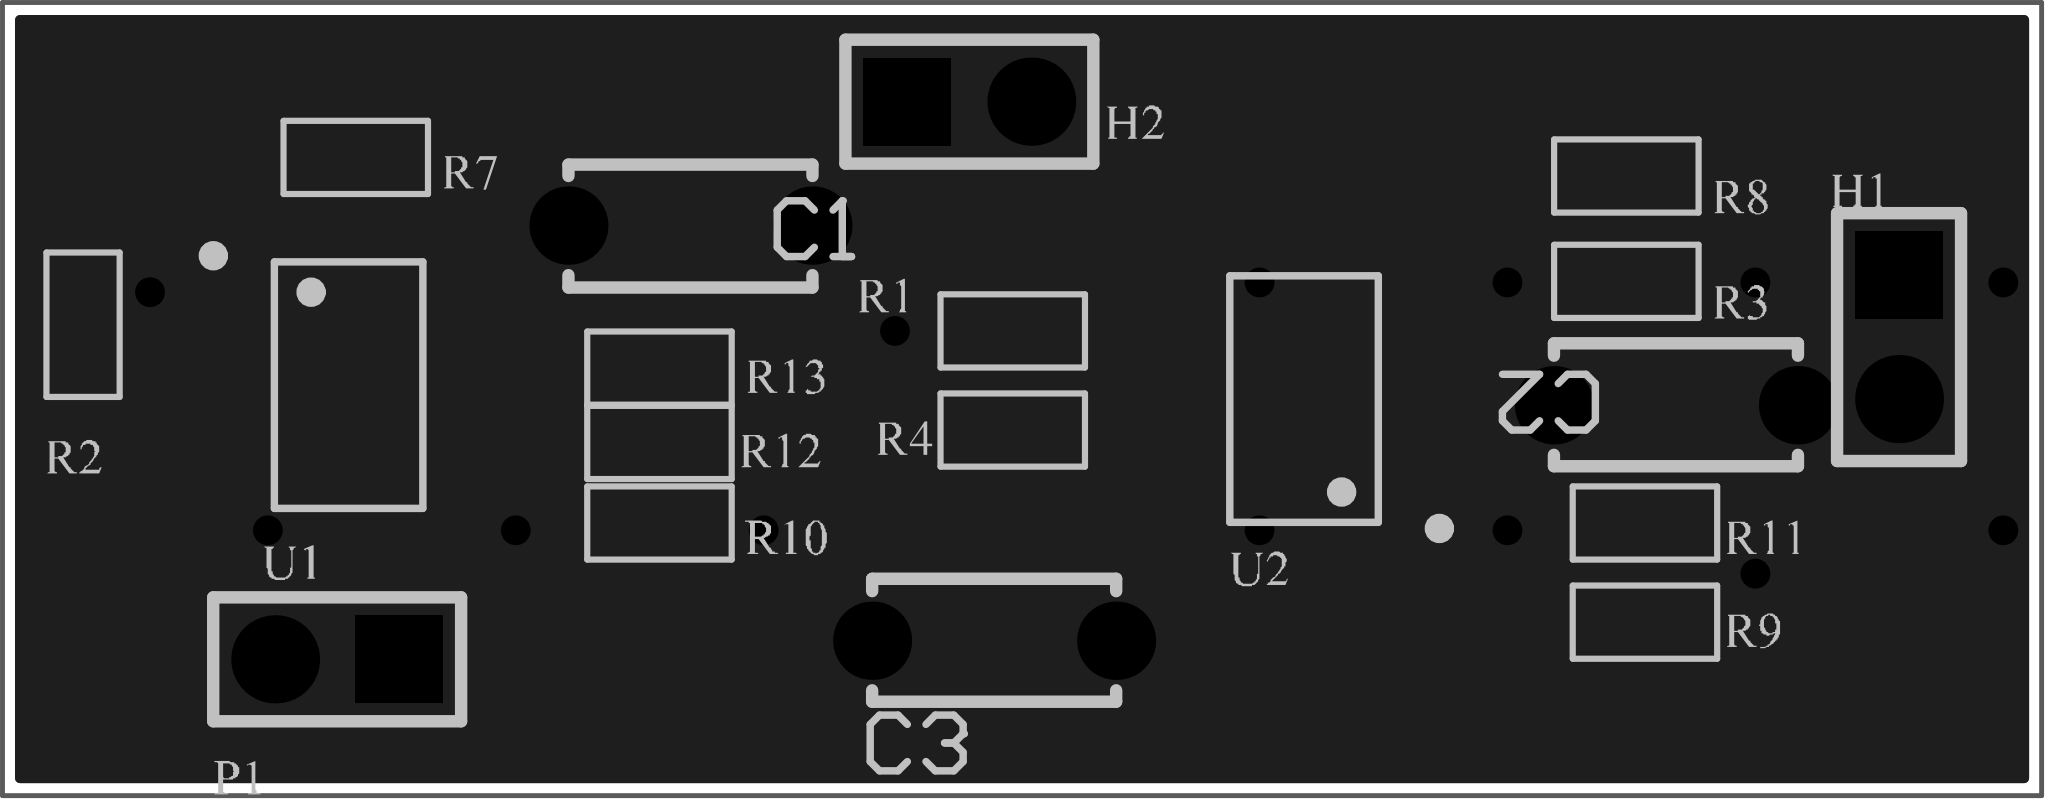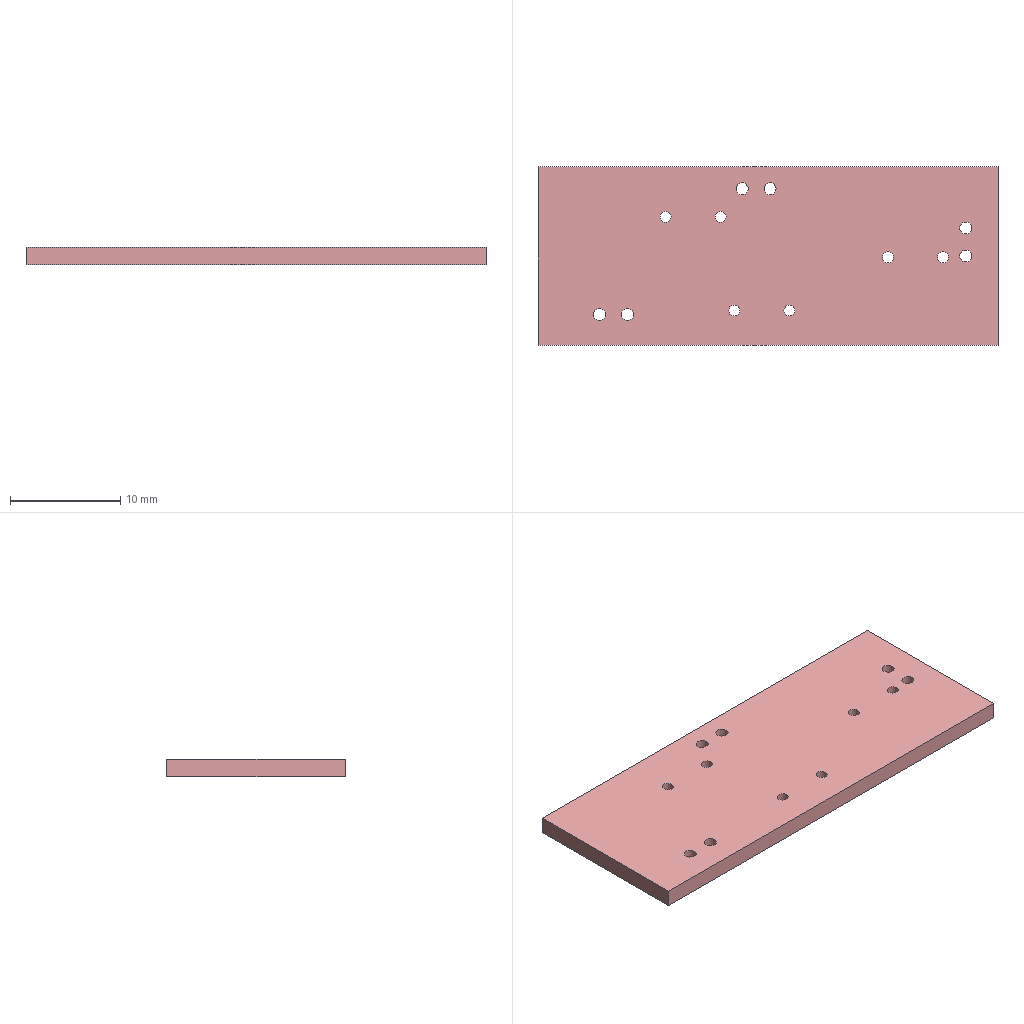Circuit board layout | Altium Designer | box 41.8 x 16.3 x 1.6 mm
Layer stack:
# Altium Designer layer stack of  (unit mm; dielectric type: 0 none, 1 core, 2 prepreg, 3 surface material)
index,name,kind,layer,copper_thickness_mm,dielectric_type,dielectric_thickness_mm,dielectric_material,dielectric_constant
0,Top Paste Mask Layer,other,,,,,,
1,Top Silkscreen Layer,other,,,,,,
2,Top Solder Mask Layer,dielectric,,,3,0.01,,3.3
3,Top Layer,copper,Top Layer,0.035,,,,
4,Dielectric1,dielectric,,,3,1.51,FR4,4.5
5,Bottom Layer,copper,Bottom Layer,0.035,,,,
6,Bottom Solder Mask Layer,dielectric,,,3,0.01,,3.3
7,Bottom Silkscreen Layer,other,,,,,,
8,Bottom Paste Mask Layer,other,,,,,,
# drill layer pairs: low layer,high layer
drill_pair,Top Layer,Bottom Layer
Part placement:
Designator,Comment,Layer,Footprint,Center-X(mm),Center-Y(mm),Rotation
H1,,TopLayer,HDR-TH_2P-P2.54-V-M-1,116.078,88.011,270
H2,,TopLayer,HDR-TH_2P-P2.54-V-M-1,97.028,92.837,0
P1,Header 2,TopLayer,HDR-TH_2P-P2.54-V-M-1,84.074,81.407,180
R1,10K,TopLayer,R0603_SMD-CRCW060327R0FKEA,97.917,88.138,180
R2,10K,TopLayer,R0603_SMD-CRCW060327R0FKEA,78.867,88.265,90
R3,1.22K,TopLayer,R0603_SMD-CRCW060327R0FKEA,110.49,89.154,180
R4,10K,TopLayer,R0603_SMD-CRCW060327R0FKEA,97.917,86.106,180
R7,100,TopLayer,R0603_SMD-CRCW060327R0FKEA,84.455,91.694,180
R8,1.22K,TopLayer,R0603_SMD-CRCW060327R0FKEA,110.49,91.313,0
R9,4.7K,TopLayer,R0603_SMD-CRCW060327R0FKEA,110.871,82.169,0
R10,10K,TopLayer,R0603_SMD-CRCW060327R0FKEA,90.678,84.201,0
R11,4.7K,TopLayer,R0603_SMD-CRCW060327R0FKEA,110.871,84.201,180
R12,10K,TopLayer,R0603_SMD-CRCW060327R0FKEA,90.678,85.852,180
R13,10K,TopLayer,R0603_SMD-CRCW060327R0FKEA,90.678,87.376,180
U1,AD8652ARZ,TopLayer,SOIC-8_L4.9-W3.9-P1.27-LS6.0-BL,84.309,87.027,270
U2,AD8652ARZ,TopLayer,SOIC-8_L4.9-W3.9-P1.27-LS6.0-BL,103.886,86.741,90
C1,Cap,TopLayer,CAP-TH_L5.0-W2.5-P5.00-D1.0,91.313,90.297,0
C2,Cap,TopLayer,CAP-TH_L5.0-W2.5-P5.00-D1.0,111.506,86.614,180
C3,Cap,TopLayer,CAP-TH_L5.0-W2.5-P5.00-D1.0,97.536,81.788,180
Pad and via stacks:
# Altium Designer via and pad stacks of  (unit mm). Each distinct definition once, with the count of objects using it.
# via: kind,start_layer,end_layer,hole_mm,diameter_mm,mode(0 simple;1 top-mid-bottom;2 full stack),diameter_per_layer,count,example_net
# pad: kind,layer,hole_mm,hole_type(0 round;1 square;2 slot),plating,top_size,top_shape(1 round;2 rect;3 octagon;9 rounded rect),mid_size,bottom_size,mode,footprint,size_per_layer,count,example
pad,Multi-Layer,1.1,0,plated,1.8x1.8,1,1.8x1.8,1.8x1.8,0,HDR-TH_2P-P2.54-V-M-1,,3,H1.2
pad,Multi-Layer,1.1,0,plated,1.8x1.8,2,1.8x1.8,1.8x1.8,0,HDR-TH_2P-P2.54-V-M-1,,3,H1.1
pad,Multi-Layer,1,0,plated,1.6x1.6,1,1.6x1.6,1.6x1.6,0,CAP-TH_L5.0-W2.5-P5.00-D1.0,,6,C1.1
pad,Top Layer,0,0,plated,0.75x1,2,0.75x1,0.75x1,0,R0603_SMD-CRCW060327R0FKEA,,22,R1.1
pad,Top Layer,0,0,plated,0.588x2.045,1,0.588x2.045,0.588x2.045,0,SOIC-8_L4.9-W3.9-P1.27-LS6.0-BL,,16,U1.5
via,Top Layer,Bottom Layer,0.3048,0.61,0,,13,$2N38
Copper pours:
name,layer,net,type(0 solid;1 hatched;2 none)
Top Layer-GND,Top Layer,GND,0
Bottom Layer-GND,Bottom Layer,GND,0